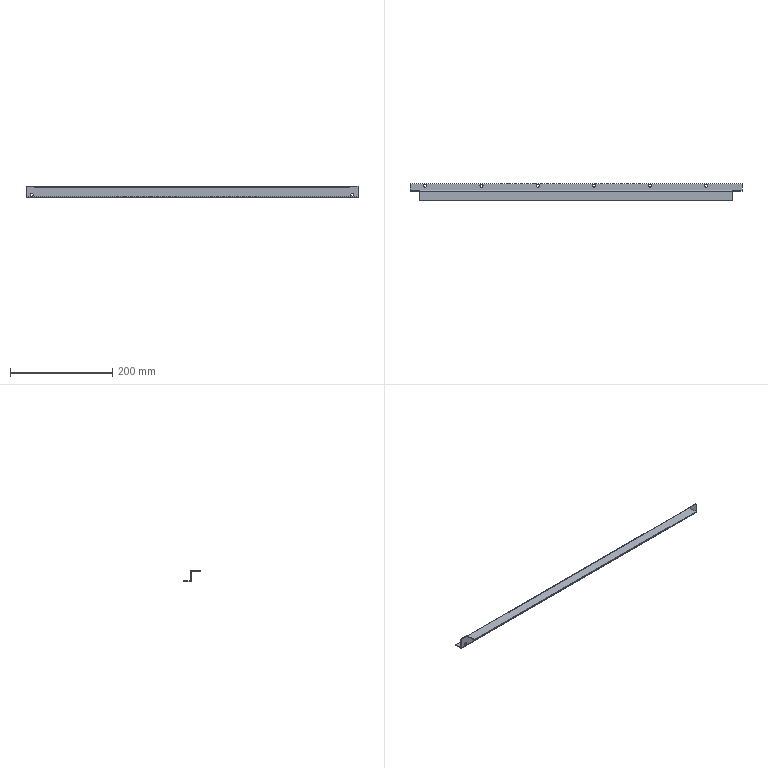Part | STEP file | Left Door Frame 2 | 1 solid | 38 faces | box 650 x 33 x 22 mm | volume 65954 mm3 | cylinder 22 | plane 16 | commonest cylinder face diameters 6 x16 0.2 x2 0.4 x2 4.2 x2
STEP:
#1=CARTESIAN_POINT('',(561.257,-2.,-4.111));
#2=VERTEX_POINT('',#1);
#3=CARTESIAN_POINT('',(561.257,-2.,1.889));
#4=VERTEX_POINT('',#3);
#5=CARTESIAN_POINT('',(561.257,-2.,-1.111));
#6=DIRECTION('',(0.,1.,0.));
#7=DIRECTION('',(0.,0.,1.));
#8=AXIS2_PLACEMENT_3D('',#5,#6,#7);
#9=CIRCLE('',#8,3.);
#10=EDGE_CURVE('',#2,#4,#9,.T.);
#11=ORIENTED_EDGE('',*,*,#10,.F.);
#12=CARTESIAN_POINT('',(561.257,0.,-4.111));
#13=VERTEX_POINT('',#12);
#14=CARTESIAN_POINT('',(561.257,-10.,-4.111));
#15=DIRECTION('',(0.,1.,0.));
#16=VECTOR('',#15,1000.);
#17=LINE('',#14,#16);
#18=EDGE_CURVE('',#2,#13,#17,.T.);
#19=ORIENTED_EDGE('',*,*,#18,.T.);
#20=CARTESIAN_POINT('',(561.257,0.,1.889));
#21=VERTEX_POINT('',#20);
#22=CARTESIAN_POINT('',(561.257,0.,-1.111));
#23=DIRECTION('',(0.,-1.,0.));
#24=DIRECTION('',(0.,0.,1.));
#25=AXIS2_PLACEMENT_3D('',#22,#23,#24);
#26=CIRCLE('',#25,3.);
#27=EDGE_CURVE('',#21,#13,#26,.T.);
#28=ORIENTED_EDGE('',*,*,#27,.F.);
#29=CARTESIAN_POINT('',(561.257,-10.,1.889));
#30=DIRECTION('',(0.,1.,0.));
#31=VECTOR('',#30,1000.);
#32=LINE('',#29,#31);
#33=EDGE_CURVE('',#4,#21,#32,.T.);
#34=ORIENTED_EDGE('',*,*,#33,.F.);
#35=EDGE_LOOP('',(#11,#19,#28,#34));
#36=FACE_OUTER_BOUND('',#35,.T.);
#37=CARTESIAN_POINT('',(561.257,-10.,-1.111));
#38=DIRECTION('',(0.,1.,0.));
#39=DIRECTION('',(0.,0.,1.));
#40=AXIS2_PLACEMENT_3D('',#37,#38,#39);
#41=CYLINDRICAL_SURFACE('',#40,3.);
#42=ADVANCED_FACE('',(#36),#41,.F.);
#43=CARTESIAN_POINT('',(-66.743,-2.,-4.111));
#44=VERTEX_POINT('',#43);
#45=CARTESIAN_POINT('',(-66.743,-2.,1.889));
#46=VERTEX_POINT('',#45);
#47=CARTESIAN_POINT('',(-66.743,-2.,-1.111));
#48=DIRECTION('',(0.,1.,0.));
#49=DIRECTION('',(0.,0.,1.));
#50=AXIS2_PLACEMENT_3D('',#47,#48,#49);
#51=CIRCLE('',#50,3.);
#52=EDGE_CURVE('',#44,#46,#51,.T.);
#53=ORIENTED_EDGE('',*,*,#52,.F.);
#54=CARTESIAN_POINT('',(-66.743,0.,-4.111));
#55=VERTEX_POINT('',#54);
#56=CARTESIAN_POINT('',(-66.743,-10.,-4.111));
#57=DIRECTION('',(0.,1.,0.));
#58=VECTOR('',#57,1000.);
#59=LINE('',#56,#58);
#60=EDGE_CURVE('',#44,#55,#59,.T.);
#61=ORIENTED_EDGE('',*,*,#60,.T.);
#62=CARTESIAN_POINT('',(-66.743,0.,1.889));
#63=VERTEX_POINT('',#62);
#64=CARTESIAN_POINT('',(-66.743,0.,-1.111));
#65=DIRECTION('',(0.,-1.,0.));
#66=DIRECTION('',(0.,0.,1.));
#67=AXIS2_PLACEMENT_3D('',#64,#65,#66);
#68=CIRCLE('',#67,3.);
#69=EDGE_CURVE('',#63,#55,#68,.T.);
#70=ORIENTED_EDGE('',*,*,#69,.F.);
#71=CARTESIAN_POINT('',(-66.743,-10.,1.889));
#72=DIRECTION('',(0.,1.,0.));
#73=VECTOR('',#72,1000.);
#74=LINE('',#71,#73);
#75=EDGE_CURVE('',#46,#63,#74,.T.);
#76=ORIENTED_EDGE('',*,*,#75,.F.);
#77=EDGE_LOOP('',(#53,#61,#70,#76));
#78=FACE_OUTER_BOUND('',#77,.T.);
#79=CARTESIAN_POINT('',(-66.743,-10.,-1.111));
#80=DIRECTION('',(0.,1.,0.));
#81=DIRECTION('',(0.,0.,1.));
#82=AXIS2_PLACEMENT_3D('',#79,#80,#81);
#83=CYLINDRICAL_SURFACE('',#82,3.);
#84=ADVANCED_FACE('',(#78),#83,.F.);
#85=CARTESIAN_POINT('',(-50.743,9.,-7.111));
#86=VERTEX_POINT('',#85);
#87=CARTESIAN_POINT('',(-44.743,9.,-7.111));
#88=VERTEX_POINT('',#87);
#89=CARTESIAN_POINT('',(-47.743,9.,-7.111));
#90=DIRECTION('',(0.,0.,1.));
#91=DIRECTION('',(1.,0.,0.));
#92=AXIS2_PLACEMENT_3D('',#89,#90,#91);
#93=CIRCLE('',#92,3.);
#94=EDGE_CURVE('',#86,#88,#93,.T.);
#95=ORIENTED_EDGE('',*,*,#94,.F.);
#96=CARTESIAN_POINT('',(-50.743,9.,-5.111));
#97=VERTEX_POINT('',#96);
#98=CARTESIAN_POINT('',(-50.743,9.,-15.111));
#99=DIRECTION('',(0.,0.,1.));
#100=VECTOR('',#99,1000.);
#101=LINE('',#98,#100);
#102=EDGE_CURVE('',#86,#97,#101,.T.);
#103=ORIENTED_EDGE('',*,*,#102,.T.);
#104=CARTESIAN_POINT('',(-44.743,9.,-5.111));
#105=VERTEX_POINT('',#104);
#106=CARTESIAN_POINT('',(-47.743,9.,-5.111));
#107=DIRECTION('',(0.,0.,-1.));
#108=DIRECTION('',(1.,0.,0.));
#109=AXIS2_PLACEMENT_3D('',#106,#107,#108);
#110=CIRCLE('',#109,3.);
#111=EDGE_CURVE('',#105,#97,#110,.T.);
#112=ORIENTED_EDGE('',*,*,#111,.F.);
#113=CARTESIAN_POINT('',(-44.743,9.,-15.111));
#114=DIRECTION('',(0.,0.,1.));
#115=VECTOR('',#114,1000.);
#116=LINE('',#113,#115);
#117=EDGE_CURVE('',#88,#105,#116,.T.);
#118=ORIENTED_EDGE('',*,*,#117,.F.);
#119=EDGE_LOOP('',(#95,#103,#112,#118));
#120=FACE_OUTER_BOUND('',#119,.T.);
#121=CARTESIAN_POINT('',(-47.743,9.,-15.111));
#122=DIRECTION('',(0.,0.,1.));
#123=DIRECTION('',(1.,0.,0.));
#124=AXIS2_PLACEMENT_3D('',#121,#122,#123);
#125=CYLINDRICAL_SURFACE('',#124,3.);
#126=ADVANCED_FACE('',(#120),#125,.F.);
#127=CARTESIAN_POINT('',(59.257,9.,-7.111));
#128=VERTEX_POINT('',#127);
#129=CARTESIAN_POINT('',(65.257,9.,-7.111));
#130=VERTEX_POINT('',#129);
#131=CARTESIAN_POINT('',(62.257,9.,-7.111));
#132=DIRECTION('',(0.,0.,1.));
#133=DIRECTION('',(1.,0.,0.));
#134=AXIS2_PLACEMENT_3D('',#131,#132,#133);
#135=CIRCLE('',#134,3.);
#136=EDGE_CURVE('',#128,#130,#135,.T.);
#137=ORIENTED_EDGE('',*,*,#136,.F.);
#138=CARTESIAN_POINT('',(59.257,9.,-5.111));
#139=VERTEX_POINT('',#138);
#140=CARTESIAN_POINT('',(59.257,9.,-15.111));
#141=DIRECTION('',(0.,0.,1.));
#142=VECTOR('',#141,1000.);
#143=LINE('',#140,#142);
#144=EDGE_CURVE('',#128,#139,#143,.T.);
#145=ORIENTED_EDGE('',*,*,#144,.T.);
#146=CARTESIAN_POINT('',(65.257,9.,-5.111));
#147=VERTEX_POINT('',#146);
#148=CARTESIAN_POINT('',(62.257,9.,-5.111));
#149=DIRECTION('',(0.,0.,-1.));
#150=DIRECTION('',(1.,0.,0.));
#151=AXIS2_PLACEMENT_3D('',#148,#149,#150);
#152=CIRCLE('',#151,3.);
#153=EDGE_CURVE('',#147,#139,#152,.T.);
#154=ORIENTED_EDGE('',*,*,#153,.F.);
#155=CARTESIAN_POINT('',(65.257,9.,-15.111));
#156=DIRECTION('',(0.,0.,1.));
#157=VECTOR('',#156,1000.);
#158=LINE('',#155,#157);
#159=EDGE_CURVE('',#130,#147,#158,.T.);
#160=ORIENTED_EDGE('',*,*,#159,.F.);
#161=EDGE_LOOP('',(#137,#145,#154,#160));
#162=FACE_OUTER_BOUND('',#161,.T.);
#163=CARTESIAN_POINT('',(62.257,9.,-15.111));
#164=DIRECTION('',(0.,0.,1.));
#165=DIRECTION('',(1.,0.,0.));
#166=AXIS2_PLACEMENT_3D('',#163,#164,#165);
#167=CYLINDRICAL_SURFACE('',#166,3.);
#168=ADVANCED_FACE('',(#162),#167,.F.);
#169=CARTESIAN_POINT('',(169.257,9.,-7.111));
#170=VERTEX_POINT('',#169);
#171=CARTESIAN_POINT('',(175.257,9.,-7.111));
#172=VERTEX_POINT('',#171);
#173=CARTESIAN_POINT('',(172.257,9.,-7.111));
#174=DIRECTION('',(0.,0.,1.));
#175=DIRECTION('',(1.,0.,0.));
#176=AXIS2_PLACEMENT_3D('',#173,#174,#175);
#177=CIRCLE('',#176,3.);
#178=EDGE_CURVE('',#170,#172,#177,.T.);
#179=ORIENTED_EDGE('',*,*,#178,.F.);
#180=CARTESIAN_POINT('',(169.257,9.,-5.111));
#181=VERTEX_POINT('',#180);
#182=CARTESIAN_POINT('',(169.257,9.,-15.111));
#183=DIRECTION('',(0.,0.,1.));
#184=VECTOR('',#183,1000.);
#185=LINE('',#182,#184);
#186=EDGE_CURVE('',#170,#181,#185,.T.);
#187=ORIENTED_EDGE('',*,*,#186,.T.);
#188=CARTESIAN_POINT('',(175.257,9.,-5.111));
#189=VERTEX_POINT('',#188);
#190=CARTESIAN_POINT('',(172.257,9.,-5.111));
#191=DIRECTION('',(0.,0.,-1.));
#192=DIRECTION('',(1.,0.,0.));
#193=AXIS2_PLACEMENT_3D('',#190,#191,#192);
#194=CIRCLE('',#193,3.);
#195=EDGE_CURVE('',#189,#181,#194,.T.);
#196=ORIENTED_EDGE('',*,*,#195,.F.);
#197=CARTESIAN_POINT('',(175.257,9.,-15.111));
#198=DIRECTION('',(0.,0.,1.));
#199=VECTOR('',#198,1000.);
#200=LINE('',#197,#199);
#201=EDGE_CURVE('',#172,#189,#200,.T.);
#202=ORIENTED_EDGE('',*,*,#201,.F.);
#203=EDGE_LOOP('',(#179,#187,#196,#202));
#204=FACE_OUTER_BOUND('',#203,.T.);
#205=CARTESIAN_POINT('',(172.257,9.,-15.111));
#206=DIRECTION('',(0.,0.,1.));
#207=DIRECTION('',(1.,0.,0.));
#208=AXIS2_PLACEMENT_3D('',#205,#206,#207);
#209=CYLINDRICAL_SURFACE('',#208,3.);
#210=ADVANCED_FACE('',(#204),#209,.F.);
#211=CARTESIAN_POINT('',(279.257,9.,-7.111));
#212=VERTEX_POINT('',#211);
#213=CARTESIAN_POINT('',(285.257,9.,-7.111));
#214=VERTEX_POINT('',#213);
#215=CARTESIAN_POINT('',(282.257,9.,-7.111));
#216=DIRECTION('',(0.,0.,1.));
#217=DIRECTION('',(1.,0.,0.));
#218=AXIS2_PLACEMENT_3D('',#215,#216,#217);
#219=CIRCLE('',#218,3.);
#220=EDGE_CURVE('',#212,#214,#219,.T.);
#221=ORIENTED_EDGE('',*,*,#220,.F.);
#222=CARTESIAN_POINT('',(279.257,9.,-5.111));
#223=VERTEX_POINT('',#222);
#224=CARTESIAN_POINT('',(279.257,9.,-15.111));
#225=DIRECTION('',(0.,0.,1.));
#226=VECTOR('',#225,1000.);
#227=LINE('',#224,#226);
#228=EDGE_CURVE('',#212,#223,#227,.T.);
#229=ORIENTED_EDGE('',*,*,#228,.T.);
#230=CARTESIAN_POINT('',(285.257,9.,-5.111));
#231=VERTEX_POINT('',#230);
#232=CARTESIAN_POINT('',(282.257,9.,-5.111));
#233=DIRECTION('',(0.,0.,-1.));
#234=DIRECTION('',(1.,0.,0.));
#235=AXIS2_PLACEMENT_3D('',#232,#233,#234);
#236=CIRCLE('',#235,3.);
#237=EDGE_CURVE('',#231,#223,#236,.T.);
#238=ORIENTED_EDGE('',*,*,#237,.F.);
#239=CARTESIAN_POINT('',(285.257,9.,-15.111));
#240=DIRECTION('',(0.,0.,1.));
#241=VECTOR('',#240,1000.);
#242=LINE('',#239,#241);
#243=EDGE_CURVE('',#214,#231,#242,.T.);
#244=ORIENTED_EDGE('',*,*,#243,.F.);
#245=EDGE_LOOP('',(#221,#229,#238,#244));
#246=FACE_OUTER_BOUND('',#245,.T.);
#247=CARTESIAN_POINT('',(282.257,9.,-15.111));
#248=DIRECTION('',(0.,0.,1.));
#249=DIRECTION('',(1.,0.,0.));
#250=AXIS2_PLACEMENT_3D('',#247,#248,#249);
#251=CYLINDRICAL_SURFACE('',#250,3.);
#252=ADVANCED_FACE('',(#246),#251,.F.);
#253=CARTESIAN_POINT('',(389.257,9.,-7.111));
#254=VERTEX_POINT('',#253);
#255=CARTESIAN_POINT('',(395.257,9.,-7.111));
#256=VERTEX_POINT('',#255);
#257=CARTESIAN_POINT('',(392.257,9.,-7.111));
#258=DIRECTION('',(0.,0.,1.));
#259=DIRECTION('',(1.,0.,0.));
#260=AXIS2_PLACEMENT_3D('',#257,#258,#259);
#261=CIRCLE('',#260,3.);
#262=EDGE_CURVE('',#254,#256,#261,.T.);
#263=ORIENTED_EDGE('',*,*,#262,.F.);
#264=CARTESIAN_POINT('',(389.257,9.,-5.111));
#265=VERTEX_POINT('',#264);
#266=CARTESIAN_POINT('',(389.257,9.,-15.111));
#267=DIRECTION('',(0.,0.,1.));
#268=VECTOR('',#267,1000.);
#269=LINE('',#266,#268);
#270=EDGE_CURVE('',#254,#265,#269,.T.);
#271=ORIENTED_EDGE('',*,*,#270,.T.);
#272=CARTESIAN_POINT('',(395.257,9.,-5.111));
#273=VERTEX_POINT('',#272);
#274=CARTESIAN_POINT('',(392.257,9.,-5.111));
#275=DIRECTION('',(0.,0.,-1.));
#276=DIRECTION('',(1.,0.,0.));
#277=AXIS2_PLACEMENT_3D('',#274,#275,#276);
#278=CIRCLE('',#277,3.);
#279=EDGE_CURVE('',#273,#265,#278,.T.);
#280=ORIENTED_EDGE('',*,*,#279,.F.);
#281=CARTESIAN_POINT('',(395.257,9.,-15.111));
#282=DIRECTION('',(0.,0.,1.));
#283=VECTOR('',#282,1000.);
#284=LINE('',#281,#283);
#285=EDGE_CURVE('',#256,#273,#284,.T.);
#286=ORIENTED_EDGE('',*,*,#285,.F.);
#287=EDGE_LOOP('',(#263,#271,#280,#286));
#288=FACE_OUTER_BOUND('',#287,.T.);
#289=CARTESIAN_POINT('',(392.257,9.,-15.111));
#290=DIRECTION('',(0.,0.,1.));
#291=DIRECTION('',(1.,0.,0.));
#292=AXIS2_PLACEMENT_3D('',#289,#290,#291);
#293=CYLINDRICAL_SURFACE('',#292,3.);
#294=ADVANCED_FACE('',(#288),#293,.F.);
#295=CARTESIAN_POINT('',(499.257,9.,-7.111));
#296=VERTEX_POINT('',#295);
#297=CARTESIAN_POINT('',(505.257,9.,-7.111));
#298=VERTEX_POINT('',#297);
#299=CARTESIAN_POINT('',(502.257,9.,-7.111));
#300=DIRECTION('',(0.,0.,1.));
#301=DIRECTION('',(1.,0.,0.));
#302=AXIS2_PLACEMENT_3D('',#299,#300,#301);
#303=CIRCLE('',#302,3.);
#304=EDGE_CURVE('',#296,#298,#303,.T.);
#305=ORIENTED_EDGE('',*,*,#304,.F.);
#306=CARTESIAN_POINT('',(499.257,9.,-5.111));
#307=VERTEX_POINT('',#306);
#308=CARTESIAN_POINT('',(499.257,9.,-15.111));
#309=DIRECTION('',(0.,0.,1.));
#310=VECTOR('',#309,1000.);
#311=LINE('',#308,#310);
#312=EDGE_CURVE('',#296,#307,#311,.T.);
#313=ORIENTED_EDGE('',*,*,#312,.T.);
#314=CARTESIAN_POINT('',(505.257,9.,-5.111));
#315=VERTEX_POINT('',#314);
#316=CARTESIAN_POINT('',(502.257,9.,-5.111));
#317=DIRECTION('',(0.,0.,-1.));
#318=DIRECTION('',(1.,0.,0.));
#319=AXIS2_PLACEMENT_3D('',#316,#317,#318);
#320=CIRCLE('',#319,3.);
#321=EDGE_CURVE('',#315,#307,#320,.T.);
#322=ORIENTED_EDGE('',*,*,#321,.F.);
#323=CARTESIAN_POINT('',(505.257,9.,-15.111));
#324=DIRECTION('',(0.,0.,1.));
#325=VECTOR('',#324,1000.);
#326=LINE('',#323,#325);
#327=EDGE_CURVE('',#298,#315,#326,.T.);
#328=ORIENTED_EDGE('',*,*,#327,.F.);
#329=EDGE_LOOP('',(#305,#313,#322,#328));
#330=FACE_OUTER_BOUND('',#329,.T.);
#331=CARTESIAN_POINT('',(502.257,9.,-15.111));
#332=DIRECTION('',(0.,0.,1.));
#333=DIRECTION('',(1.,0.,0.));
#334=AXIS2_PLACEMENT_3D('',#331,#332,#333);
#335=CYLINDRICAL_SURFACE('',#334,3.);
#336=ADVANCED_FACE('',(#330),#335,.F.);
#337=CARTESIAN_POINT('',(572.257,0.,-5.011));
#338=VERTEX_POINT('',#337);
#339=CARTESIAN_POINT('',(-77.743,0.,-5.011));
#340=VERTEX_POINT('',#339);
#341=CARTESIAN_POINT('',(0.,0.,-5.011));
#342=DIRECTION('',(-1.,0.,0.));
#343=VECTOR('',#342,1000.);
#344=LINE('',#341,#343);
#345=EDGE_CURVE('',#338,#340,#344,.T.);
#346=ORIENTED_EDGE('',*,*,#345,.T.);
#347=CARTESIAN_POINT('',(-77.743,0.,14.889));
#348=VERTEX_POINT('',#347);
#349=CARTESIAN_POINT('',(-77.743,0.,0.));
#350=DIRECTION('',(0.,0.,1.));
#351=VECTOR('',#350,1000.);
#352=LINE('',#349,#351);
#353=EDGE_CURVE('',#340,#348,#352,.T.);
#354=ORIENTED_EDGE('',*,*,#353,.T.);
#355=CARTESIAN_POINT('',(-60.143,0.,14.889));
#356=VERTEX_POINT('',#355);
#357=CARTESIAN_POINT('',(0.,0.,14.889));
#358=DIRECTION('',(1.,0.,0.));
#359=VECTOR('',#358,1000.);
#360=LINE('',#357,#359);
#361=EDGE_CURVE('',#348,#356,#360,.T.);
#362=ORIENTED_EDGE('',*,*,#361,.T.);
#363=CARTESIAN_POINT('',(-60.143,0.,12.389));
#364=VERTEX_POINT('',#363);
#365=CARTESIAN_POINT('',(-60.143,0.,0.));
#366=DIRECTION('',(0.,0.,-1.));
#367=VECTOR('',#366,1000.);
#368=LINE('',#365,#367);
#369=EDGE_CURVE('',#356,#364,#368,.T.);
#370=ORIENTED_EDGE('',*,*,#369,.T.);
#371=CARTESIAN_POINT('',(-59.743,0.,12.389));
#372=VERTEX_POINT('',#371);
#373=CARTESIAN_POINT('',(-59.943,0.,12.389));
#374=DIRECTION('',(0.,-1.,0.));
#375=DIRECTION('',(0.,0.,1.));
#376=AXIS2_PLACEMENT_3D('',#373,#374,#375);
#377=CIRCLE('',#376,0.2);
#378=EDGE_CURVE('',#364,#372,#377,.T.);
#379=ORIENTED_EDGE('',*,*,#378,.T.);
#380=CARTESIAN_POINT('',(-59.743,0.,12.789));
#381=VERTEX_POINT('',#380);
#382=CARTESIAN_POINT('',(-59.743,0.,12.389));
#383=DIRECTION('',(0.,0.,-1.));
#384=VECTOR('',#383,1000.);
#385=LINE('',#382,#384);
#386=EDGE_CURVE('',#381,#372,#385,.T.);
#387=ORIENTED_EDGE('',*,*,#386,.F.);
#388=CARTESIAN_POINT('',(554.257,0.,12.789));
#389=VERTEX_POINT('',#388);
#390=CARTESIAN_POINT('',(0.,0.,12.789));
#391=DIRECTION('',(1.,0.,0.));
#392=VECTOR('',#391,1000.);
#393=LINE('',#390,#392);
#394=EDGE_CURVE('',#381,#389,#393,.T.);
#395=ORIENTED_EDGE('',*,*,#394,.T.);
#396=CARTESIAN_POINT('',(554.257,0.,12.389));
#397=VERTEX_POINT('',#396);
#398=CARTESIAN_POINT('',(554.257,0.,12.789));
#399=DIRECTION('',(0.,0.,1.));
#400=VECTOR('',#399,1000.);
#401=LINE('',#398,#400);
#402=EDGE_CURVE('',#397,#389,#401,.T.);
#403=ORIENTED_EDGE('',*,*,#402,.F.);
#404=CARTESIAN_POINT('',(554.657,0.,12.389));
#405=VERTEX_POINT('',#404);
#406=CARTESIAN_POINT('',(554.457,0.,12.389));
#407=DIRECTION('',(0.,-1.,0.));
#408=DIRECTION('',(0.,0.,1.));
#409=AXIS2_PLACEMENT_3D('',#406,#407,#408);
#410=CIRCLE('',#409,0.2);
#411=EDGE_CURVE('',#397,#405,#410,.T.);
#412=ORIENTED_EDGE('',*,*,#411,.T.);
#413=CARTESIAN_POINT('',(554.657,0.,14.889));
#414=VERTEX_POINT('',#413);
#415=CARTESIAN_POINT('',(554.657,0.,0.));
#416=DIRECTION('',(0.,0.,1.));
#417=VECTOR('',#416,1000.);
#418=LINE('',#415,#417);
#419=EDGE_CURVE('',#405,#414,#418,.T.);
#420=ORIENTED_EDGE('',*,*,#419,.T.);
#421=CARTESIAN_POINT('',(572.257,0.,14.889));
#422=VERTEX_POINT('',#421);
#423=CARTESIAN_POINT('',(0.,0.,14.889));
#424=DIRECTION('',(1.,0.,0.));
#425=VECTOR('',#424,1000.);
#426=LINE('',#423,#425);
#427=EDGE_CURVE('',#414,#422,#426,.T.);
#428=ORIENTED_EDGE('',*,*,#427,.T.);
#429=CARTESIAN_POINT('',(572.257,0.,0.));
#430=DIRECTION('',(0.,0.,-1.));
#431=VECTOR('',#430,1000.);
#432=LINE('',#429,#431);
#433=EDGE_CURVE('',#422,#338,#432,.T.);
#434=ORIENTED_EDGE('',*,*,#433,.T.);
#435=EDGE_LOOP('',(#346,#354,#362,#370,#379,#387,#395,#403,#412,#420,#428,#434));
#436=FACE_OUTER_BOUND('',#435,.T.);
#437=ORIENTED_EDGE('',*,*,#27,.T.);
#438=CARTESIAN_POINT('',(561.257,0.,-1.111));
#439=DIRECTION('',(0.,-1.,0.));
#440=DIRECTION('',(0.,0.,1.));
#441=AXIS2_PLACEMENT_3D('',#438,#439,#440);
#442=CIRCLE('',#441,3.);
#443=EDGE_CURVE('',#13,#21,#442,.T.);
#444=ORIENTED_EDGE('',*,*,#443,.T.);
#445=EDGE_LOOP('',(#437,#444));
#446=FACE_BOUND('',#445,.T.);
#447=ORIENTED_EDGE('',*,*,#69,.T.);
#448=CARTESIAN_POINT('',(-66.743,0.,-1.111));
#449=DIRECTION('',(0.,-1.,0.));
#450=DIRECTION('',(0.,0.,1.));
#451=AXIS2_PLACEMENT_3D('',#448,#449,#450);
#452=CIRCLE('',#451,3.);
#453=EDGE_CURVE('',#55,#63,#452,.T.);
#454=ORIENTED_EDGE('',*,*,#453,.T.);
#455=EDGE_LOOP('',(#447,#454));
#456=FACE_BOUND('',#455,.T.);
#457=CARTESIAN_POINT('',(0.,0.,0.));
#458=DIRECTION('',(0.,1.,0.));
#459=DIRECTION('',(0.,0.,1.));
#460=AXIS2_PLACEMENT_3D('',#457,#458,#459);
#461=PLANE('',#460);
#462=ADVANCED_FACE('',(#436,#446,#456),#461,.T.);
#463=CARTESIAN_POINT('',(-77.743,-2.,-5.011));
#464=VERTEX_POINT('',#463);
#465=CARTESIAN_POINT('',(-77.743,-2.,14.889));
#466=VERTEX_POINT('',#465);
#467=CARTESIAN_POINT('',(-77.743,-2.,-7.111));
#468=DIRECTION('',(0.,0.,1.));
#469=VECTOR('',#468,1000.);
#470=LINE('',#467,#469);
#471=EDGE_CURVE('',#464,#466,#470,.T.);
#472=ORIENTED_EDGE('',*,*,#471,.T.);
#473=CARTESIAN_POINT('',(-77.743,-2.,14.889));
#474=DIRECTION('',(0.,1.,0.));
#475=VECTOR('',#474,1000.);
#476=LINE('',#473,#475);
#477=EDGE_CURVE('',#466,#348,#476,.T.);
#478=ORIENTED_EDGE('',*,*,#477,.T.);
#479=ORIENTED_EDGE('',*,*,#353,.F.);
#480=CARTESIAN_POINT('',(-77.743,0.1,-5.111));
#481=VERTEX_POINT('',#480);
#482=CARTESIAN_POINT('',(-77.743,0.1,-5.011));
#483=DIRECTION('',(1.,0.,0.));
#484=DIRECTION('',(0.,-1.,0.));
#485=AXIS2_PLACEMENT_3D('',#482,#483,#484);
#486=CIRCLE('',#485,0.1);
#487=EDGE_CURVE('',#340,#481,#486,.T.);
#488=ORIENTED_EDGE('',*,*,#487,.T.);
#489=CARTESIAN_POINT('',(-77.743,13.,-5.111));
#490=VERTEX_POINT('',#489);
#491=CARTESIAN_POINT('',(-77.743,0.,-5.111));
#492=DIRECTION('',(0.,-1.,0.));
#493=VECTOR('',#492,1000.);
#494=LINE('',#491,#493);
#495=EDGE_CURVE('',#490,#481,#494,.T.);
#496=ORIENTED_EDGE('',*,*,#495,.F.);
#497=CARTESIAN_POINT('',(-77.743,13.,-7.111));
#498=VERTEX_POINT('',#497);
#499=CARTESIAN_POINT('',(-77.743,13.,-7.111));
#500=DIRECTION('',(0.,0.,1.));
#501=VECTOR('',#500,1000.);
#502=LINE('',#499,#501);
#503=EDGE_CURVE('',#498,#490,#502,.T.);
#504=ORIENTED_EDGE('',*,*,#503,.F.);
#505=CARTESIAN_POINT('',(-77.743,0.1,-7.111));
#506=VERTEX_POINT('',#505);
#507=CARTESIAN_POINT('',(-77.743,13.,-7.111));
#508=DIRECTION('',(0.,1.,0.));
#509=VECTOR('',#508,1000.);
#510=LINE('',#507,#509);
#511=EDGE_CURVE('',#506,#498,#510,.T.);
#512=ORIENTED_EDGE('',*,*,#511,.F.);
#513=CARTESIAN_POINT('',(-77.743,0.1,-5.011));
#514=DIRECTION('',(1.,0.,0.));
#515=DIRECTION('',(0.,-1.,0.));
#516=AXIS2_PLACEMENT_3D('',#513,#514,#515);
#517=CIRCLE('',#516,2.1);
#518=EDGE_CURVE('',#464,#506,#517,.T.);
#519=ORIENTED_EDGE('',*,*,#518,.F.);
#520=EDGE_LOOP('',(#472,#478,#479,#488,#496,#504,#512,#519));
#521=FACE_OUTER_BOUND('',#520,.T.);
#522=CARTESIAN_POINT('',(-77.743,-2.,-7.111));
#523=DIRECTION('',(-1.,0.,0.));
#524=DIRECTION('',(0.,0.,1.));
#525=AXIS2_PLACEMENT_3D('',#522,#523,#524);
#526=PLANE('',#525);
#527=ADVANCED_FACE('',(#521),#526,.T.);
#528=CARTESIAN_POINT('',(572.257,0.1,-5.111));
#529=VERTEX_POINT('',#528);
#530=CARTESIAN_POINT('',(572.257,0.1,-5.011));
#531=DIRECTION('',(-1.,0.,0.));
#532=DIRECTION('',(0.,-1.,0.));
#533=AXIS2_PLACEMENT_3D('',#530,#531,#532);
#534=CIRCLE('',#533,0.1);
#535=EDGE_CURVE('',#529,#338,#534,.T.);
#536=ORIENTED_EDGE('',*,*,#535,.F.);
#537=CARTESIAN_POINT('',(-77.743,0.1,-5.111));
#538=DIRECTION('',(1.,0.,0.));
#539=VECTOR('',#538,1000.);
#540=LINE('',#537,#539);
#541=EDGE_CURVE('',#481,#529,#540,.T.);
#542=ORIENTED_EDGE('',*,*,#541,.F.);
#543=ORIENTED_EDGE('',*,*,#487,.F.);
#544=ORIENTED_EDGE('',*,*,#345,.F.);
#545=EDGE_LOOP('',(#536,#542,#543,#544));
#546=FACE_OUTER_BOUND('',#545,.T.);
#547=CARTESIAN_POINT('',(-77.743,0.1,-5.011));
#548=DIRECTION('',(-1.,0.,0.));
#549=DIRECTION('',(0.,-1.,0.));
#550=AXIS2_PLACEMENT_3D('',#547,#548,#549);
#551=CYLINDRICAL_SURFACE('',#550,0.1);
#552=ADVANCED_FACE('',(#546),#551,.F.);
#553=CARTESIAN_POINT('',(572.257,-2.,14.889));
#554=VERTEX_POINT('',#553);
#555=CARTESIAN_POINT('',(572.257,-2.,14.889));
#556=DIRECTION('',(0.,-1.,0.));
#557=VECTOR('',#556,1000.);
#558=LINE('',#555,#557);
#559=EDGE_CURVE('',#422,#554,#558,.T.);
#560=ORIENTED_EDGE('',*,*,#559,.T.);
#561=CARTESIAN_POINT('',(572.257,-2.,-5.011));
#562=VERTEX_POINT('',#561);
#563=CARTESIAN_POINT('',(572.257,-2.,-7.111));
#564=DIRECTION('',(0.,0.,-1.));
#565=VECTOR('',#564,1000.);
#566=LINE('',#563,#565);
#567=EDGE_CURVE('',#554,#562,#566,.T.);
#568=ORIENTED_EDGE('',*,*,#567,.T.);
#569=CARTESIAN_POINT('',(572.257,0.1,-7.111));
#570=VERTEX_POINT('',#569);
#571=CARTESIAN_POINT('',(572.257,0.1,-5.011));
#572=DIRECTION('',(1.,0.,0.));
#573=DIRECTION('',(0.,-1.,0.));
#574=AXIS2_PLACEMENT_3D('',#571,#572,#573);
#575=CIRCLE('',#574,2.1);
#576=EDGE_CURVE('',#562,#570,#575,.T.);
#577=ORIENTED_EDGE('',*,*,#576,.T.);
#578=CARTESIAN_POINT('',(572.257,13.,-7.111));
#579=VERTEX_POINT('',#578);
#580=CARTESIAN_POINT('',(572.257,0.,-7.111));
#581=DIRECTION('',(0.,-1.,0.));
#582=VECTOR('',#581,1000.);
#583=LINE('',#580,#582);
#584=EDGE_CURVE('',#579,#570,#583,.T.);
#585=ORIENTED_EDGE('',*,*,#584,.F.);
#586=CARTESIAN_POINT('',(572.257,13.,-5.111));
#587=VERTEX_POINT('',#586);
#588=CARTESIAN_POINT('',(572.257,13.,-7.111));
#589=DIRECTION('',(0.,0.,1.));
#590=VECTOR('',#589,1000.);
#591=LINE('',#588,#590);
#592=EDGE_CURVE('',#579,#587,#591,.T.);
#593=ORIENTED_EDGE('',*,*,#592,.T.);
#594=CARTESIAN_POINT('',(572.257,0.,-5.111));
#595=DIRECTION('',(0.,1.,0.));
#596=VECTOR('',#595,1000.);
#597=LINE('',#594,#596);
#598=EDGE_CURVE('',#529,#587,#597,.T.);
#599=ORIENTED_EDGE('',*,*,#598,.F.);
#600=ORIENTED_EDGE('',*,*,#535,.T.);
#601=ORIENTED_EDGE('',*,*,#433,.F.);
#602=EDGE_LOOP('',(#560,#568,#577,#585,#593,#599,#600,#601));
#603=FACE_OUTER_BOUND('',#602,.T.);
#604=CARTESIAN_POINT('',(572.257,-2.,-7.111));
#605=DIRECTION('',(1.,0.,0.));
#606=DIRECTION('',(0.,0.,-1.));
#607=AXIS2_PLACEMENT_3D('',#604,#605,#606);
#608=PLANE('',#607);
#609=ADVANCED_FACE('',(#603),#608,.T.);
#610=CARTESIAN_POINT('',(554.657,-2.,14.889));
#611=VERTEX_POINT('',#610);
#612=CARTESIAN_POINT('',(-77.743,-2.,14.889));
#613=DIRECTION('',(1.,0.,0.));
#614=VECTOR('',#613,1000.);
#615=LINE('',#612,#614);
#616=EDGE_CURVE('',#611,#554,#615,.T.);
#617=ORIENTED_EDGE('',*,*,#616,.T.);
#618=ORIENTED_EDGE('',*,*,#559,.F.);
#619=ORIENTED_EDGE('',*,*,#427,.F.);
#620=CARTESIAN_POINT('',(554.657,-2.,14.889));
#621=DIRECTION('',(0.,-1.,0.));
#622=VECTOR('',#621,1000.);
#623=LINE('',#620,#622);
#624=EDGE_CURVE('',#414,#611,#623,.T.);
#625=ORIENTED_EDGE('',*,*,#624,.T.);
#626=EDGE_LOOP('',(#617,#618,#619,#625));
#627=FACE_OUTER_BOUND('',#626,.T.);
#628=CARTESIAN_POINT('',(-77.743,-2.,14.889));
#629=DIRECTION('',(0.,0.,1.));
#630=DIRECTION('',(1.,0.,0.));
#631=AXIS2_PLACEMENT_3D('',#628,#629,#630);
#632=PLANE('',#631);
#633=ADVANCED_FACE('',(#627),#632,.T.);
#634=CARTESIAN_POINT('',(554.657,-2.,12.389));
#635=VERTEX_POINT('',#634);
#636=CARTESIAN_POINT('',(554.657,-2.,12.389));
#637=DIRECTION('',(0.,0.,1.));
#638=VECTOR('',#637,1000.);
#639=LINE('',#636,#638);
#640=EDGE_CURVE('',#635,#611,#639,.T.);
#641=ORIENTED_EDGE('',*,*,#640,.T.);
#642=ORIENTED_EDGE('',*,*,#624,.F.);
#643=ORIENTED_EDGE('',*,*,#419,.F.);
#644=CARTESIAN_POINT('',(554.657,-2.,12.389));
#645=DIRECTION('',(0.,-1.,0.));
#646=VECTOR('',#645,1000.);
#647=LINE('',#644,#646);
#648=EDGE_CURVE('',#405,#635,#647,.T.);
#649=ORIENTED_EDGE('',*,*,#648,.T.);
#650=EDGE_LOOP('',(#641,#642,#643,#649));
#651=FACE_OUTER_BOUND('',#650,.T.);
#652=CARTESIAN_POINT('',(554.657,-2.,12.389));
#653=DIRECTION('',(-1.,0.,0.));
#654=DIRECTION('',(0.,0.,1.));
#655=AXIS2_PLACEMENT_3D('',#652,#653,#654);
#656=PLANE('',#655);
#657=ADVANCED_FACE('',(#651),#656,.T.);
#658=CARTESIAN_POINT('',(-59.743,-2.1,14.889));
#659=VERTEX_POINT('',#658);
#660=CARTESIAN_POINT('',(554.257,-2.1,14.889));
#661=VERTEX_POINT('',#660);
#662=CARTESIAN_POINT('',(-59.743,-2.1,14.889));
#663=DIRECTION('',(1.,0.,0.));
#664=VECTOR('',#663,1000.);
#665=LINE('',#662,#664);
#666=EDGE_CURVE('',#659,#661,#665,.T.);
#667=ORIENTED_EDGE('',*,*,#666,.T.);
#668=CARTESIAN_POINT('',(554.257,-2.1,12.789));
#669=DIRECTION('',(-1.,0.,0.));
#670=DIRECTION('',(0.,0.,1.));
#671=AXIS2_PLACEMENT_3D('',#668,#669,#670);
#672=CIRCLE('',#671,2.1);
#673=EDGE_CURVE('',#661,#389,#672,.T.);
#674=ORIENTED_EDGE('',*,*,#673,.T.);
#675=ORIENTED_EDGE('',*,*,#394,.F.);
#676=CARTESIAN_POINT('',(-59.743,-2.1,12.789));
#677=DIRECTION('',(1.,0.,0.));
#678=DIRECTION('',(0.,0.,1.));
#679=AXIS2_PLACEMENT_3D('',#676,#677,#678);
#680=CIRCLE('',#679,2.1);
#681=EDGE_CURVE('',#381,#659,#680,.T.);
#682=ORIENTED_EDGE('',*,*,#681,.T.);
#683=EDGE_LOOP('',(#667,#674,#675,#682));
#684=FACE_OUTER_BOUND('',#683,.T.);
#685=CARTESIAN_POINT('',(-59.743,-2.1,12.789));
#686=DIRECTION('',(-1.,0.,0.));
#687=DIRECTION('',(0.,0.,1.));
#688=AXIS2_PLACEMENT_3D('',#685,#686,#687);
#689=CYLINDRICAL_SURFACE('',#688,2.1);
#690=ADVANCED_FACE('',(#684),#689,.T.);
#691=CARTESIAN_POINT('',(-60.143,-2.,14.889));
#692=VERTEX_POINT('',#691);
#693=CARTESIAN_POINT('',(-60.143,-2.,12.389));
#694=VERTEX_POINT('',#693);
#695=CARTESIAN_POINT('',(-60.143,-2.,14.889));
#696=DIRECTION('',(0.,0.,-1.));
#697=VECTOR('',#696,1000.);
#698=LINE('',#695,#697);
#699=EDGE_CURVE('',#692,#694,#698,.T.);
#700=ORIENTED_EDGE('',*,*,#699,.T.);
#701=CARTESIAN_POINT('',(-60.143,-2.,12.389));
#702=DIRECTION('',(0.,1.,0.));
#703=VECTOR('',#702,1000.);
#704=LINE('',#701,#703);
#705=EDGE_CURVE('',#694,#364,#704,.T.);
#706=ORIENTED_EDGE('',*,*,#705,.T.);
#707=ORIENTED_EDGE('',*,*,#369,.F.);
#708=CARTESIAN_POINT('',(-60.143,-2.,14.889));
#709=DIRECTION('',(0.,-1.,0.));
#710=VECTOR('',#709,1000.);
#711=LINE('',#708,#710);
#712=EDGE_CURVE('',#356,#692,#711,.T.);
#713=ORIENTED_EDGE('',*,*,#712,.T.);
#714=EDGE_LOOP('',(#700,#706,#707,#713));
#715=FACE_OUTER_BOUND('',#714,.T.);
#716=CARTESIAN_POINT('',(-60.143,-2.,14.889));
#717=DIRECTION('',(1.,0.,0.));
#718=DIRECTION('',(0.,0.,-1.));
#719=AXIS2_PLACEMENT_3D('',#716,#717,#718);
#720=PLANE('',#719);
#721=ADVANCED_FACE('',(#715),#720,.T.);
#722=ORIENTED_EDGE('',*,*,#361,.F.);
#723=ORIENTED_EDGE('',*,*,#477,.F.);
#724=CARTESIAN_POINT('',(-77.743,-2.,14.889));
#725=DIRECTION('',(1.,0.,0.));
#726=VECTOR('',#725,1000.);
#727=LINE('',#724,#726);
#728=EDGE_CURVE('',#466,#692,#727,.T.);
#729=ORIENTED_EDGE('',*,*,#728,.T.);
#730=ORIENTED_EDGE('',*,*,#712,.F.);
#731=EDGE_LOOP('',(#722,#723,#729,#730));
#732=FACE_OUTER_BOUND('',#731,.T.);
#733=CARTESIAN_POINT('',(-77.743,-2.,14.889));
#734=DIRECTION('',(0.,0.,1.));
#735=DIRECTION('',(1.,0.,0.));
#736=AXIS2_PLACEMENT_3D('',#733,#734,#735);
#737=PLANE('',#736);
#738=ADVANCED_FACE('',(#732),#737,.T.);
#739=ORIENTED_EDGE('',*,*,#18,.F.);
#740=CARTESIAN_POINT('',(561.257,-2.,-1.111));
#741=DIRECTION('',(0.,1.,0.));
#742=DIRECTION('',(0.,0.,1.));
#743=AXIS2_PLACEMENT_3D('',#740,#741,#742);
#744=CIRCLE('',#743,3.);
#745=EDGE_CURVE('',#4,#2,#744,.T.);
#746=ORIENTED_EDGE('',*,*,#745,.F.);
#747=ORIENTED_EDGE('',*,*,#33,.T.);
#748=ORIENTED_EDGE('',*,*,#443,.F.);
#749=EDGE_LOOP('',(#739,#746,#747,#748));
#750=FACE_OUTER_BOUND('',#749,.T.);
#751=CARTESIAN_POINT('',(561.257,-10.,-1.111));
#752=DIRECTION('',(0.,1.,0.));
#753=DIRECTION('',(0.,0.,1.));
#754=AXIS2_PLACEMENT_3D('',#751,#752,#753);
#755=CYLINDRICAL_SURFACE('',#754,3.);
#756=ADVANCED_FACE('',(#750),#755,.F.);
#757=ORIENTED_EDGE('',*,*,#60,.F.);
#758=CARTESIAN_POINT('',(-66.743,-2.,-1.111));
#759=DIRECTION('',(0.,1.,0.));
#760=DIRECTION('',(0.,0.,1.));
#761=AXIS2_PLACEMENT_3D('',#758,#759,#760);
#762=CIRCLE('',#761,3.);
#763=EDGE_CURVE('',#46,#44,#762,.T.);
#764=ORIENTED_EDGE('',*,*,#763,.F.);
#765=ORIENTED_EDGE('',*,*,#75,.T.);
#766=ORIENTED_EDGE('',*,*,#453,.F.);
#767=EDGE_LOOP('',(#757,#764,#765,#766));
#768=FACE_OUTER_BOUND('',#767,.T.);
#769=CARTESIAN_POINT('',(-66.743,-10.,-1.111));
#770=DIRECTION('',(0.,1.,0.));
#771=DIRECTION('',(0.,0.,1.));
#772=AXIS2_PLACEMENT_3D('',#769,#770,#771);
#773=CYLINDRICAL_SURFACE('',#772,3.);
#774=ADVANCED_FACE('',(#768),#773,.F.);
#775=ORIENTED_EDGE('',*,*,#728,.F.);
#776=ORIENTED_EDGE('',*,*,#471,.F.);
#777=CARTESIAN_POINT('',(0.,-2.,-5.011));
#778=DIRECTION('',(-1.,0.,0.));
#779=VECTOR('',#778,1000.);
#780=LINE('',#777,#779);
#781=EDGE_CURVE('',#562,#464,#780,.T.);
#782=ORIENTED_EDGE('',*,*,#781,.F.);
#783=ORIENTED_EDGE('',*,*,#567,.F.);
#784=ORIENTED_EDGE('',*,*,#616,.F.);
#785=ORIENTED_EDGE('',*,*,#640,.F.);
#786=CARTESIAN_POINT('',(554.257,-2.,12.389));
#787=VERTEX_POINT('',#786);
#788=CARTESIAN_POINT('',(554.457,-2.,12.389));
#789=DIRECTION('',(0.,-1.,0.));
#790=DIRECTION('',(0.,0.,1.));
#791=AXIS2_PLACEMENT_3D('',#788,#789,#790);
#792=CIRCLE('',#791,0.2);
#793=EDGE_CURVE('',#787,#635,#792,.T.);
#794=ORIENTED_EDGE('',*,*,#793,.F.);
#795=CARTESIAN_POINT('',(554.257,-2.,12.789));
#796=VERTEX_POINT('',#795);
#797=CARTESIAN_POINT('',(554.257,-2.,12.789));
#798=DIRECTION('',(0.,0.,-1.));
#799=VECTOR('',#798,1000.);
#800=LINE('',#797,#799);
#801=EDGE_CURVE('',#796,#787,#800,.T.);
#802=ORIENTED_EDGE('',*,*,#801,.F.);
#803=CARTESIAN_POINT('',(-59.743,-2.,12.789));
#804=VERTEX_POINT('',#803);
#805=CARTESIAN_POINT('',(0.,-2.,12.789));
#806=DIRECTION('',(1.,0.,0.));
#807=VECTOR('',#806,1000.);
#808=LINE('',#805,#807);
#809=EDGE_CURVE('',#804,#796,#808,.T.);
#810=ORIENTED_EDGE('',*,*,#809,.F.);
#811=CARTESIAN_POINT('',(-59.743,-2.,12.389));
#812=VERTEX_POINT('',#811);
#813=CARTESIAN_POINT('',(-59.743,-2.,12.389));
#814=DIRECTION('',(0.,0.,1.));
#815=VECTOR('',#814,1000.);
#816=LINE('',#813,#815);
#817=EDGE_CURVE('',#812,#804,#816,.T.);
#818=ORIENTED_EDGE('',*,*,#817,.F.);
#819=CARTESIAN_POINT('',(-59.943,-2.,12.389));
#820=DIRECTION('',(0.,-1.,0.));
#821=DIRECTION('',(0.,0.,1.));
#822=AXIS2_PLACEMENT_3D('',#819,#820,#821);
#823=CIRCLE('',#822,0.2);
#824=EDGE_CURVE('',#694,#812,#823,.T.);
#825=ORIENTED_EDGE('',*,*,#824,.F.);
#826=ORIENTED_EDGE('',*,*,#699,.F.);
#827=EDGE_LOOP('',(#775,#776,#782,#783,#784,#785,#794,#802,#810,#818,#825,#826));
#828=FACE_OUTER_BOUND('',#827,.T.);
#829=ORIENTED_EDGE('',*,*,#745,.T.);
#830=ORIENTED_EDGE('',*,*,#10,.T.);
#831=EDGE_LOOP('',(#829,#830));
#832=FACE_BOUND('',#831,.T.);
#833=ORIENTED_EDGE('',*,*,#763,.T.);
#834=ORIENTED_EDGE('',*,*,#52,.T.);
#835=EDGE_LOOP('',(#833,#834));
#836=FACE_BOUND('',#835,.T.);
#837=CARTESIAN_POINT('',(0.,-2.,0.));
#838=DIRECTION('',(0.,1.,0.));
#839=DIRECTION('',(0.,0.,1.));
#840=AXIS2_PLACEMENT_3D('',#837,#838,#839);
#841=PLANE('',#840);
#842=ADVANCED_FACE('',(#828,#832,#836),#841,.F.);
#843=ORIENTED_EDGE('',*,*,#598,.T.);
#844=CARTESIAN_POINT('',(0.,13.,-5.111));
#845=DIRECTION('',(-1.,0.,0.));
#846=VECTOR('',#845,1000.);
#847=LINE('',#844,#846);
#848=EDGE_CURVE('',#587,#490,#847,.T.);
#849=ORIENTED_EDGE('',*,*,#848,.T.);
#850=ORIENTED_EDGE('',*,*,#495,.T.);
#851=ORIENTED_EDGE('',*,*,#541,.T.);
#852=EDGE_LOOP('',(#843,#849,#850,#851));
#853=FACE_OUTER_BOUND('',#852,.T.);
#854=ORIENTED_EDGE('',*,*,#111,.T.);
#855=CARTESIAN_POINT('',(-47.743,9.,-5.111));
#856=DIRECTION('',(0.,0.,-1.));
#857=DIRECTION('',(1.,0.,0.));
#858=AXIS2_PLACEMENT_3D('',#855,#856,#857);
#859=CIRCLE('',#858,3.);
#860=EDGE_CURVE('',#97,#105,#859,.T.);
#861=ORIENTED_EDGE('',*,*,#860,.T.);
#862=EDGE_LOOP('',(#854,#861));
#863=FACE_BOUND('',#862,.T.);
#864=ORIENTED_EDGE('',*,*,#153,.T.);
#865=CARTESIAN_POINT('',(62.257,9.,-5.111));
#866=DIRECTION('',(0.,0.,-1.));
#867=DIRECTION('',(1.,0.,0.));
#868=AXIS2_PLACEMENT_3D('',#865,#866,#867);
#869=CIRCLE('',#868,3.);
#870=EDGE_CURVE('',#139,#147,#869,.T.);
#871=ORIENTED_EDGE('',*,*,#870,.T.);
#872=EDGE_LOOP('',(#864,#871));
#873=FACE_BOUND('',#872,.T.);
#874=ORIENTED_EDGE('',*,*,#195,.T.);
#875=CARTESIAN_POINT('',(172.257,9.,-5.111));
#876=DIRECTION('',(0.,0.,-1.));
#877=DIRECTION('',(1.,0.,0.));
#878=AXIS2_PLACEMENT_3D('',#875,#876,#877);
#879=CIRCLE('',#878,3.);
#880=EDGE_CURVE('',#181,#189,#879,.T.);
#881=ORIENTED_EDGE('',*,*,#880,.T.);
#882=EDGE_LOOP('',(#874,#881));
#883=FACE_BOUND('',#882,.T.);
#884=ORIENTED_EDGE('',*,*,#237,.T.);
#885=CARTESIAN_POINT('',(282.257,9.,-5.111));
#886=DIRECTION('',(0.,0.,-1.));
#887=DIRECTION('',(1.,0.,0.));
#888=AXIS2_PLACEMENT_3D('',#885,#886,#887);
#889=CIRCLE('',#888,3.);
#890=EDGE_CURVE('',#223,#231,#889,.T.);
#891=ORIENTED_EDGE('',*,*,#890,.T.);
#892=EDGE_LOOP('',(#884,#891));
#893=FACE_BOUND('',#892,.T.);
#894=ORIENTED_EDGE('',*,*,#279,.T.);
#895=CARTESIAN_POINT('',(392.257,9.,-5.111));
#896=DIRECTION('',(0.,0.,-1.));
#897=DIRECTION('',(1.,0.,0.));
#898=AXIS2_PLACEMENT_3D('',#895,#896,#897);
#899=CIRCLE('',#898,3.);
#900=EDGE_CURVE('',#265,#273,#899,.T.);
#901=ORIENTED_EDGE('',*,*,#900,.T.);
#902=EDGE_LOOP('',(#894,#901));
#903=FACE_BOUND('',#902,.T.);
#904=ORIENTED_EDGE('',*,*,#321,.T.);
#905=CARTESIAN_POINT('',(502.257,9.,-5.111));
#906=DIRECTION('',(0.,0.,-1.));
#907=DIRECTION('',(1.,0.,0.));
#908=AXIS2_PLACEMENT_3D('',#905,#906,#907);
#909=CIRCLE('',#908,3.);
#910=EDGE_CURVE('',#307,#315,#909,.T.);
#911=ORIENTED_EDGE('',*,*,#910,.T.);
#912=EDGE_LOOP('',(#904,#911));
#913=FACE_BOUND('',#912,.T.);
#914=CARTESIAN_POINT('',(0.,0.,-5.111));
#915=DIRECTION('',(0.,0.,1.));
#916=DIRECTION('',(0.,-1.,0.));
#917=AXIS2_PLACEMENT_3D('',#914,#915,#916);
#918=PLANE('',#917);
#919=ADVANCED_FACE('',(#853,#863,#873,#883,#893,#903,#913),#918,.T.);
#920=CARTESIAN_POINT('',(554.257,-2.,12.389));
#921=DIRECTION('',(0.,1.,0.));
#922=VECTOR('',#921,1000.);
#923=LINE('',#920,#922);
#924=EDGE_CURVE('',#787,#397,#923,.T.);
#925=ORIENTED_EDGE('',*,*,#924,.F.);
#926=ORIENTED_EDGE('',*,*,#793,.T.);
#927=ORIENTED_EDGE('',*,*,#648,.F.);
#928=ORIENTED_EDGE('',*,*,#411,.F.);
#929=EDGE_LOOP('',(#925,#926,#927,#928));
#930=FACE_OUTER_BOUND('',#929,.T.);
#931=CARTESIAN_POINT('',(554.457,-2.,12.389));
#932=DIRECTION('',(0.,1.,0.));
#933=DIRECTION('',(0.,0.,1.));
#934=AXIS2_PLACEMENT_3D('',#931,#932,#933);
#935=CYLINDRICAL_SURFACE('',#934,0.2);
#936=ADVANCED_FACE('',(#930),#935,.F.);
#937=CARTESIAN_POINT('',(554.257,-2.1,12.889));
#938=VERTEX_POINT('',#937);
#939=CARTESIAN_POINT('',(554.257,-2.1,12.789));
#940=DIRECTION('',(-1.,0.,0.));
#941=DIRECTION('',(0.,0.,1.));
#942=AXIS2_PLACEMENT_3D('',#939,#940,#941);
#943=CIRCLE('',#942,0.1);
#944=EDGE_CURVE('',#938,#796,#943,.T.);
#945=ORIENTED_EDGE('',*,*,#944,.T.);
#946=ORIENTED_EDGE('',*,*,#801,.T.);
#947=ORIENTED_EDGE('',*,*,#924,.T.);
#948=ORIENTED_EDGE('',*,*,#402,.T.);
#949=ORIENTED_EDGE('',*,*,#673,.F.);
#950=CARTESIAN_POINT('',(554.257,-20.,14.889));
#951=VERTEX_POINT('',#950);
#952=CARTESIAN_POINT('',(554.257,0.,14.889));
#953=DIRECTION('',(0.,1.,0.));
#954=VECTOR('',#953,1000.);
#955=LINE('',#952,#954);
#956=EDGE_CURVE('',#951,#661,#955,.T.);
#957=ORIENTED_EDGE('',*,*,#956,.F.);
#958=CARTESIAN_POINT('',(554.257,-20.,12.889));
#959=VERTEX_POINT('',#958);
#960=CARTESIAN_POINT('',(554.257,-20.,14.889));
#961=DIRECTION('',(0.,0.,-1.));
#962=VECTOR('',#961,1000.);
#963=LINE('',#960,#962);
#964=EDGE_CURVE('',#951,#959,#963,.T.);
#965=ORIENTED_EDGE('',*,*,#964,.T.);
#966=CARTESIAN_POINT('',(554.257,-20.,12.889));
#967=DIRECTION('',(0.,1.,0.));
#968=VECTOR('',#967,1000.);
#969=LINE('',#966,#968);
#970=EDGE_CURVE('',#959,#938,#969,.T.);
#971=ORIENTED_EDGE('',*,*,#970,.T.);
#972=EDGE_LOOP('',(#945,#946,#947,#948,#949,#957,#965,#971));
#973=FACE_OUTER_BOUND('',#972,.T.);
#974=CARTESIAN_POINT('',(554.257,-2.1,12.789));
#975=DIRECTION('',(1.,0.,0.));
#976=DIRECTION('',(0.,0.,-1.));
#977=AXIS2_PLACEMENT_3D('',#974,#975,#976);
#978=PLANE('',#977);
#979=ADVANCED_FACE('',(#973),#978,.T.);
#980=CARTESIAN_POINT('',(-59.743,-20.,14.889));
#981=VERTEX_POINT('',#980);
#982=CARTESIAN_POINT('',(-59.743,0.,14.889));
#983=DIRECTION('',(0.,-1.,0.));
#984=VECTOR('',#983,1000.);
#985=LINE('',#982,#984);
#986=EDGE_CURVE('',#659,#981,#985,.T.);
#987=ORIENTED_EDGE('',*,*,#986,.T.);
#988=CARTESIAN_POINT('',(0.,-20.,14.889));
#989=DIRECTION('',(1.,0.,0.));
#990=VECTOR('',#989,1000.);
#991=LINE('',#988,#990);
#992=EDGE_CURVE('',#981,#951,#991,.T.);
#993=ORIENTED_EDGE('',*,*,#992,.T.);
#994=ORIENTED_EDGE('',*,*,#956,.T.);
#995=ORIENTED_EDGE('',*,*,#666,.F.);
#996=EDGE_LOOP('',(#987,#993,#994,#995));
#997=FACE_OUTER_BOUND('',#996,.T.);
#998=CARTESIAN_POINT('',(0.,0.,14.889));
#999=DIRECTION('',(0.,0.,1.));
#1000=DIRECTION('',(0.,-1.,0.));
#1001=AXIS2_PLACEMENT_3D('',#998,#999,#1000);
#1002=PLANE('',#1001);
#1003=ADVANCED_FACE('',(#997),#1002,.T.);
#1004=CARTESIAN_POINT('',(-59.743,-2.1,12.889));
#1005=VERTEX_POINT('',#1004);
#1006=CARTESIAN_POINT('',(-59.743,-2.1,12.789));
#1007=DIRECTION('',(-1.,0.,0.));
#1008=DIRECTION('',(0.,0.,1.));
#1009=AXIS2_PLACEMENT_3D('',#1006,#1007,#1008);
#1010=CIRCLE('',#1009,0.1);
#1011=EDGE_CURVE('',#1005,#804,#1010,.T.);
#1012=ORIENTED_EDGE('',*,*,#1011,.F.);
#1013=CARTESIAN_POINT('',(-59.743,-20.,12.889));
#1014=VERTEX_POINT('',#1013);
#1015=CARTESIAN_POINT('',(-59.743,-2.,12.889));
#1016=DIRECTION('',(0.,-1.,0.));
#1017=VECTOR('',#1016,1000.);
#1018=LINE('',#1015,#1017);
#1019=EDGE_CURVE('',#1005,#1014,#1018,.T.);
#1020=ORIENTED_EDGE('',*,*,#1019,.T.);
#1021=CARTESIAN_POINT('',(-59.743,-20.,14.889));
#1022=DIRECTION('',(0.,0.,-1.));
#1023=VECTOR('',#1022,1000.);
#1024=LINE('',#1021,#1023);
#1025=EDGE_CURVE('',#981,#1014,#1024,.T.);
#1026=ORIENTED_EDGE('',*,*,#1025,.F.);
#1027=ORIENTED_EDGE('',*,*,#986,.F.);
#1028=ORIENTED_EDGE('',*,*,#681,.F.);
#1029=ORIENTED_EDGE('',*,*,#386,.T.);
#1030=CARTESIAN_POINT('',(-59.743,-2.,12.389));
#1031=DIRECTION('',(0.,-1.,0.));
#1032=VECTOR('',#1031,1000.);
#1033=LINE('',#1030,#1032);
#1034=EDGE_CURVE('',#372,#812,#1033,.T.);
#1035=ORIENTED_EDGE('',*,*,#1034,.T.);
#1036=ORIENTED_EDGE('',*,*,#817,.T.);
#1037=EDGE_LOOP('',(#1012,#1020,#1026,#1027,#1028,#1029,#1035,#1036));
#1038=FACE_OUTER_BOUND('',#1037,.T.);
#1039=CARTESIAN_POINT('',(-59.743,-2.1,12.789));
#1040=DIRECTION('',(1.,0.,0.));
#1041=DIRECTION('',(0.,0.,-1.));
#1042=AXIS2_PLACEMENT_3D('',#1039,#1040,#1041);
#1043=PLANE('',#1042);
#1044=ADVANCED_FACE('',(#1038),#1043,.F.);
#1045=ORIENTED_EDGE('',*,*,#705,.F.);
#1046=ORIENTED_EDGE('',*,*,#824,.T.);
#1047=ORIENTED_EDGE('',*,*,#1034,.F.);
#1048=ORIENTED_EDGE('',*,*,#378,.F.);
#1049=EDGE_LOOP('',(#1045,#1046,#1047,#1048));
#1050=FACE_OUTER_BOUND('',#1049,.T.);
#1051=CARTESIAN_POINT('',(-59.943,-2.,12.389));
#1052=DIRECTION('',(0.,1.,0.));
#1053=DIRECTION('',(0.,0.,1.));
#1054=AXIS2_PLACEMENT_3D('',#1051,#1052,#1053);
#1055=CYLINDRICAL_SURFACE('',#1054,0.2);
#1056=ADVANCED_FACE('',(#1050),#1055,.F.);
#1057=CARTESIAN_POINT('',(-77.743,0.1,-7.111));
#1058=DIRECTION('',(1.,0.,0.));
#1059=VECTOR('',#1058,1000.);
#1060=LINE('',#1057,#1059);
#1061=EDGE_CURVE('',#506,#570,#1060,.T.);
#1062=ORIENTED_EDGE('',*,*,#1061,.T.);
#1063=ORIENTED_EDGE('',*,*,#576,.F.);
#1064=ORIENTED_EDGE('',*,*,#781,.T.);
#1065=ORIENTED_EDGE('',*,*,#518,.T.);
#1066=EDGE_LOOP('',(#1062,#1063,#1064,#1065));
#1067=FACE_OUTER_BOUND('',#1066,.T.);
#1068=CARTESIAN_POINT('',(-77.743,0.1,-5.011));
#1069=DIRECTION('',(-1.,0.,0.));
#1070=DIRECTION('',(0.,-1.,0.));
#1071=AXIS2_PLACEMENT_3D('',#1068,#1069,#1070);
#1072=CYLINDRICAL_SURFACE('',#1071,2.1);
#1073=ADVANCED_FACE('',(#1067),#1072,.T.);
#1074=ORIENTED_EDGE('',*,*,#944,.F.);
#1075=CARTESIAN_POINT('',(-59.743,-2.1,12.889));
#1076=DIRECTION('',(1.,0.,0.));
#1077=VECTOR('',#1076,1000.);
#1078=LINE('',#1075,#1077);
#1079=EDGE_CURVE('',#1005,#938,#1078,.T.);
#1080=ORIENTED_EDGE('',*,*,#1079,.F.);
#1081=ORIENTED_EDGE('',*,*,#1011,.T.);
#1082=ORIENTED_EDGE('',*,*,#809,.T.);
#1083=EDGE_LOOP('',(#1074,#1080,#1081,#1082));
#1084=FACE_OUTER_BOUND('',#1083,.T.);
#1085=CARTESIAN_POINT('',(-59.743,-2.1,12.789));
#1086=DIRECTION('',(-1.,0.,0.));
#1087=DIRECTION('',(0.,0.,1.));
#1088=AXIS2_PLACEMENT_3D('',#1085,#1086,#1087);
#1089=CYLINDRICAL_SURFACE('',#1088,0.1);
#1090=ADVANCED_FACE('',(#1084),#1089,.F.);
#1091=ORIENTED_EDGE('',*,*,#592,.F.);
#1092=CARTESIAN_POINT('',(572.257,13.,-7.111));
#1093=DIRECTION('',(1.,0.,0.));
#1094=VECTOR('',#1093,1000.);
#1095=LINE('',#1092,#1094);
#1096=EDGE_CURVE('',#498,#579,#1095,.T.);
#1097=ORIENTED_EDGE('',*,*,#1096,.F.);
#1098=ORIENTED_EDGE('',*,*,#503,.T.);
#1099=ORIENTED_EDGE('',*,*,#848,.F.);
#1100=EDGE_LOOP('',(#1091,#1097,#1098,#1099));
#1101=FACE_OUTER_BOUND('',#1100,.T.);
#1102=CARTESIAN_POINT('',(572.257,13.,-7.111));
#1103=DIRECTION('',(0.,-1.,0.));
#1104=DIRECTION('',(0.,0.,-1.));
#1105=AXIS2_PLACEMENT_3D('',#1102,#1103,#1104);
#1106=PLANE('',#1105);
#1107=ADVANCED_FACE('',(#1101),#1106,.F.);
#1108=ORIENTED_EDGE('',*,*,#102,.F.);
#1109=CARTESIAN_POINT('',(-47.743,9.,-7.111));
#1110=DIRECTION('',(0.,0.,1.));
#1111=DIRECTION('',(1.,0.,0.));
#1112=AXIS2_PLACEMENT_3D('',#1109,#1110,#1111);
#1113=CIRCLE('',#1112,3.);
#1114=EDGE_CURVE('',#88,#86,#1113,.T.);
#1115=ORIENTED_EDGE('',*,*,#1114,.F.);
#1116=ORIENTED_EDGE('',*,*,#117,.T.);
#1117=ORIENTED_EDGE('',*,*,#860,.F.);
#1118=EDGE_LOOP('',(#1108,#1115,#1116,#1117));
#1119=FACE_OUTER_BOUND('',#1118,.T.);
#1120=CARTESIAN_POINT('',(-47.743,9.,-15.111));
#1121=DIRECTION('',(0.,0.,1.));
#1122=DIRECTION('',(1.,0.,0.));
#1123=AXIS2_PLACEMENT_3D('',#1120,#1121,#1122);
#1124=CYLINDRICAL_SURFACE('',#1123,3.);
#1125=ADVANCED_FACE('',(#1119),#1124,.F.);
#1126=ORIENTED_EDGE('',*,*,#144,.F.);
#1127=CARTESIAN_POINT('',(62.257,9.,-7.111));
#1128=DIRECTION('',(0.,0.,1.));
#1129=DIRECTION('',(1.,0.,0.));
#1130=AXIS2_PLACEMENT_3D('',#1127,#1128,#1129);
#1131=CIRCLE('',#1130,3.);
#1132=EDGE_CURVE('',#130,#128,#1131,.T.);
#1133=ORIENTED_EDGE('',*,*,#1132,.F.);
#1134=ORIENTED_EDGE('',*,*,#159,.T.);
#1135=ORIENTED_EDGE('',*,*,#870,.F.);
#1136=EDGE_LOOP('',(#1126,#1133,#1134,#1135));
#1137=FACE_OUTER_BOUND('',#1136,.T.);
#1138=CARTESIAN_POINT('',(62.257,9.,-15.111));
#1139=DIRECTION('',(0.,0.,1.));
#1140=DIRECTION('',(1.,0.,0.));
#1141=AXIS2_PLACEMENT_3D('',#1138,#1139,#1140);
#1142=CYLINDRICAL_SURFACE('',#1141,3.);
#1143=ADVANCED_FACE('',(#1137),#1142,.F.);
#1144=ORIENTED_EDGE('',*,*,#186,.F.);
#1145=CARTESIAN_POINT('',(172.257,9.,-7.111));
#1146=DIRECTION('',(0.,0.,1.));
#1147=DIRECTION('',(1.,0.,0.));
#1148=AXIS2_PLACEMENT_3D('',#1145,#1146,#1147);
#1149=CIRCLE('',#1148,3.);
#1150=EDGE_CURVE('',#172,#170,#1149,.T.);
#1151=ORIENTED_EDGE('',*,*,#1150,.F.);
#1152=ORIENTED_EDGE('',*,*,#201,.T.);
#1153=ORIENTED_EDGE('',*,*,#880,.F.);
#1154=EDGE_LOOP('',(#1144,#1151,#1152,#1153));
#1155=FACE_OUTER_BOUND('',#1154,.T.);
#1156=CARTESIAN_POINT('',(172.257,9.,-15.111));
#1157=DIRECTION('',(0.,0.,1.));
#1158=DIRECTION('',(1.,0.,0.));
#1159=AXIS2_PLACEMENT_3D('',#1156,#1157,#1158);
#1160=CYLINDRICAL_SURFACE('',#1159,3.);
#1161=ADVANCED_FACE('',(#1155),#1160,.F.);
#1162=ORIENTED_EDGE('',*,*,#228,.F.);
#1163=CARTESIAN_POINT('',(282.257,9.,-7.111));
#1164=DIRECTION('',(0.,0.,1.));
#1165=DIRECTION('',(1.,0.,0.));
#1166=AXIS2_PLACEMENT_3D('',#1163,#1164,#1165);
#1167=CIRCLE('',#1166,3.);
#1168=EDGE_CURVE('',#214,#212,#1167,.T.);
#1169=ORIENTED_EDGE('',*,*,#1168,.F.);
#1170=ORIENTED_EDGE('',*,*,#243,.T.);
#1171=ORIENTED_EDGE('',*,*,#890,.F.);
#1172=EDGE_LOOP('',(#1162,#1169,#1170,#1171));
#1173=FACE_OUTER_BOUND('',#1172,.T.);
#1174=CARTESIAN_POINT('',(282.257,9.,-15.111));
#1175=DIRECTION('',(0.,0.,1.));
#1176=DIRECTION('',(1.,0.,0.));
#1177=AXIS2_PLACEMENT_3D('',#1174,#1175,#1176);
#1178=CYLINDRICAL_SURFACE('',#1177,3.);
#1179=ADVANCED_FACE('',(#1173),#1178,.F.);
#1180=ORIENTED_EDGE('',*,*,#270,.F.);
#1181=CARTESIAN_POINT('',(392.257,9.,-7.111));
#1182=DIRECTION('',(0.,0.,1.));
#1183=DIRECTION('',(1.,0.,0.));
#1184=AXIS2_PLACEMENT_3D('',#1181,#1182,#1183);
#1185=CIRCLE('',#1184,3.);
#1186=EDGE_CURVE('',#256,#254,#1185,.T.);
#1187=ORIENTED_EDGE('',*,*,#1186,.F.);
#1188=ORIENTED_EDGE('',*,*,#285,.T.);
#1189=ORIENTED_EDGE('',*,*,#900,.F.);
#1190=EDGE_LOOP('',(#1180,#1187,#1188,#1189));
#1191=FACE_OUTER_BOUND('',#1190,.T.);
#1192=CARTESIAN_POINT('',(392.257,9.,-15.111));
#1193=DIRECTION('',(0.,0.,1.));
#1194=DIRECTION('',(1.,0.,0.));
#1195=AXIS2_PLACEMENT_3D('',#1192,#1193,#1194);
#1196=CYLINDRICAL_SURFACE('',#1195,3.);
#1197=ADVANCED_FACE('',(#1191),#1196,.F.);
#1198=ORIENTED_EDGE('',*,*,#312,.F.);
#1199=CARTESIAN_POINT('',(502.257,9.,-7.111));
#1200=DIRECTION('',(0.,0.,1.));
#1201=DIRECTION('',(1.,0.,0.));
#1202=AXIS2_PLACEMENT_3D('',#1199,#1200,#1201);
#1203=CIRCLE('',#1202,3.);
#1204=EDGE_CURVE('',#298,#296,#1203,.T.);
#1205=ORIENTED_EDGE('',*,*,#1204,.F.);
#1206=ORIENTED_EDGE('',*,*,#327,.T.);
#1207=ORIENTED_EDGE('',*,*,#910,.F.);
#1208=EDGE_LOOP('',(#1198,#1205,#1206,#1207));
#1209=FACE_OUTER_BOUND('',#1208,.T.);
#1210=CARTESIAN_POINT('',(502.257,9.,-15.111));
#1211=DIRECTION('',(0.,0.,1.));
#1212=DIRECTION('',(1.,0.,0.));
#1213=AXIS2_PLACEMENT_3D('',#1210,#1211,#1212);
#1214=CYLINDRICAL_SURFACE('',#1213,3.);
#1215=ADVANCED_FACE('',(#1209),#1214,.F.);
#1216=ORIENTED_EDGE('',*,*,#992,.F.);
#1217=ORIENTED_EDGE('',*,*,#1025,.T.);
#1218=CARTESIAN_POINT('',(-59.743,-20.,12.889));
#1219=DIRECTION('',(1.,0.,0.));
#1220=VECTOR('',#1219,1000.);
#1221=LINE('',#1218,#1220);
#1222=EDGE_CURVE('',#1014,#959,#1221,.T.);
#1223=ORIENTED_EDGE('',*,*,#1222,.T.);
#1224=ORIENTED_EDGE('',*,*,#964,.F.);
#1225=EDGE_LOOP('',(#1216,#1217,#1223,#1224));
#1226=FACE_OUTER_BOUND('',#1225,.T.);
#1227=CARTESIAN_POINT('',(-59.743,-20.,14.889));
#1228=DIRECTION('',(0.,-1.,0.));
#1229=DIRECTION('',(0.,0.,-1.));
#1230=AXIS2_PLACEMENT_3D('',#1227,#1228,#1229);
#1231=PLANE('',#1230);
#1232=ADVANCED_FACE('',(#1226),#1231,.T.);
#1233=ORIENTED_EDGE('',*,*,#511,.T.);
#1234=ORIENTED_EDGE('',*,*,#1096,.T.);
#1235=ORIENTED_EDGE('',*,*,#584,.T.);
#1236=ORIENTED_EDGE('',*,*,#1061,.F.);
#1237=EDGE_LOOP('',(#1233,#1234,#1235,#1236));
#1238=FACE_OUTER_BOUND('',#1237,.T.);
#1239=ORIENTED_EDGE('',*,*,#1114,.T.);
#1240=ORIENTED_EDGE('',*,*,#94,.T.);
#1241=EDGE_LOOP('',(#1239,#1240));
#1242=FACE_BOUND('',#1241,.T.);
#1243=ORIENTED_EDGE('',*,*,#1132,.T.);
#1244=ORIENTED_EDGE('',*,*,#136,.T.);
#1245=EDGE_LOOP('',(#1243,#1244));
#1246=FACE_BOUND('',#1245,.T.);
#1247=ORIENTED_EDGE('',*,*,#1150,.T.);
#1248=ORIENTED_EDGE('',*,*,#178,.T.);
#1249=EDGE_LOOP('',(#1247,#1248));
#1250=FACE_BOUND('',#1249,.T.);
#1251=ORIENTED_EDGE('',*,*,#1168,.T.);
#1252=ORIENTED_EDGE('',*,*,#220,.T.);
#1253=EDGE_LOOP('',(#1251,#1252));
#1254=FACE_BOUND('',#1253,.T.);
#1255=ORIENTED_EDGE('',*,*,#1186,.T.);
#1256=ORIENTED_EDGE('',*,*,#262,.T.);
#1257=EDGE_LOOP('',(#1255,#1256));
#1258=FACE_BOUND('',#1257,.T.);
#1259=ORIENTED_EDGE('',*,*,#1204,.T.);
#1260=ORIENTED_EDGE('',*,*,#304,.T.);
#1261=EDGE_LOOP('',(#1259,#1260));
#1262=FACE_BOUND('',#1261,.T.);
#1263=CARTESIAN_POINT('',(0.,0.,-7.111));
#1264=DIRECTION('',(0.,0.,1.));
#1265=DIRECTION('',(0.,-1.,0.));
#1266=AXIS2_PLACEMENT_3D('',#1263,#1264,#1265);
#1267=PLANE('',#1266);
#1268=ADVANCED_FACE('',(#1238,#1242,#1246,#1250,#1254,#1258,#1262),#1267,.F.);
#1269=ORIENTED_EDGE('',*,*,#970,.F.);
#1270=ORIENTED_EDGE('',*,*,#1222,.F.);
#1271=ORIENTED_EDGE('',*,*,#1019,.F.);
#1272=ORIENTED_EDGE('',*,*,#1079,.T.);
#1273=EDGE_LOOP('',(#1269,#1270,#1271,#1272));
#1274=FACE_OUTER_BOUND('',#1273,.T.);
#1275=CARTESIAN_POINT('',(0.,0.,12.889));
#1276=DIRECTION('',(0.,0.,1.));
#1277=DIRECTION('',(0.,-1.,0.));
#1278=AXIS2_PLACEMENT_3D('',#1275,#1276,#1277);
#1279=PLANE('',#1278);
#1280=ADVANCED_FACE('',(#1274),#1279,.F.);
#1281=CLOSED_SHELL('',(#42,#84,#126,#168,#210,#252,#294,#336,#462,#527,#552,#609,#633,#657,#690,#721,#738,#756,#774,#842,#919,#936,#979,#1003,#1044,#1056,#1073,#1090,#1107,#1125,#1143,#1161,#1179,#1197,#1215,#1232,#1268,#1280));
#1282=MANIFOLD_SOLID_BREP('',#1281);
#1283=CARTESIAN_POINT('',(0.,0.,0.));
#1284=DIRECTION('',(0.,0.,1.));
#1285=DIRECTION('',(1.,0.,0.));
#1286=AXIS2_PLACEMENT_3D('',#1283,#1284,#1285);
#1287=(LENGTH_UNIT()NAMED_UNIT(*)SI_UNIT(.MILLI.,.METRE.));
#1288=UNCERTAINTY_MEASURE_WITH_UNIT(LENGTH_MEASURE(0.00001),#1287,'','');
#1289=(NAMED_UNIT(*)PLANE_ANGLE_UNIT()SI_UNIT($,.RADIAN.));
#1290=(NAMED_UNIT(*)SI_UNIT($,.STERADIAN.)SOLID_ANGLE_UNIT());
#1291=(GEOMETRIC_REPRESENTATION_CONTEXT(3)GLOBAL_UNCERTAINTY_ASSIGNED_CONTEXT((#1288))GLOBAL_UNIT_ASSIGNED_CONTEXT((#1287,#1289,#1290))REPRESENTATION_CONTEXT('',''));
#1292=ADVANCED_BREP_SHAPE_REPRESENTATION('',(#1282,#1286),#1291);